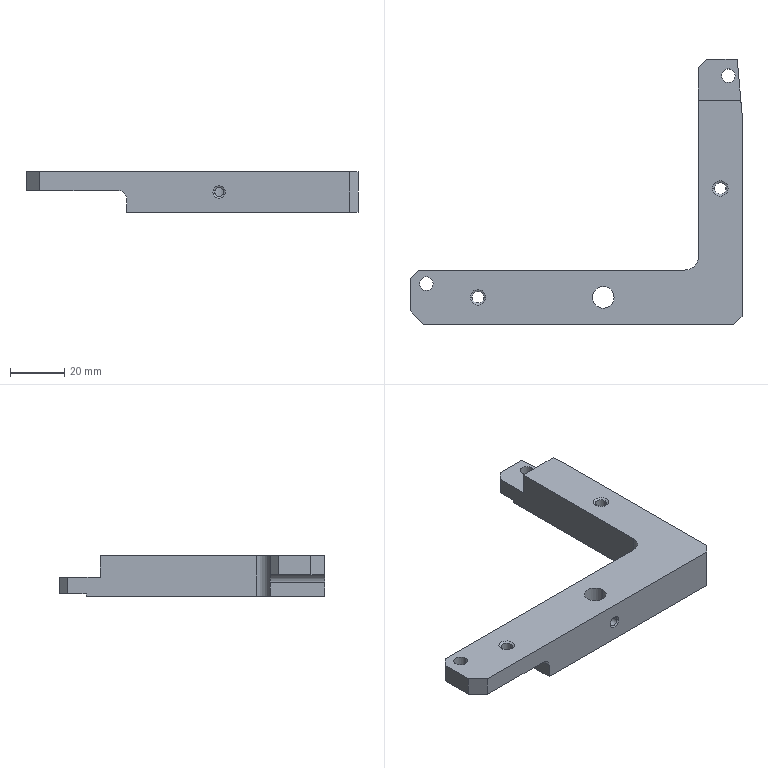Part | NX | 1 solid | 39 faces | box 122 x 97.43 x 15 mm | volume 45601 mm3 | plane 19 | cylinder 14 | cone 6 | commonest cylinder face diameters 4.2 x4 5 x4 3.3 x2 8 x2 6 x1 10 x1
STEP:
#1=CARTESIAN_POINT('',(-61.,7.,0.5));
#2=VERTEX_POINT('',#1);
#3=CARTESIAN_POINT('',(-61.,-5.,0.5));
#4=VERTEX_POINT('',#3);
#5=CARTESIAN_POINT('',(-61.,0.,0.5));
#6=DIRECTION('',(0.,-1.,0.));
#7=VECTOR('',#6,1000.);
#8=LINE('',#5,#7);
#9=EDGE_CURVE('',#2,#4,#8,.T.);
#10=ORIENTED_EDGE('',*,*,#9,.F.);
#11=CARTESIAN_POINT('',(-58.,10.,0.5));
#12=VERTEX_POINT('',#11);
#13=CARTESIAN_POINT('',(-68.,0.,0.5));
#14=DIRECTION('',(-0.7071,-0.7071,0.));
#15=VECTOR('',#14,1000.);
#16=LINE('',#13,#15);
#17=EDGE_CURVE('',#12,#2,#16,.T.);
#18=ORIENTED_EDGE('',*,*,#17,.F.);
#19=CARTESIAN_POINT('',(-27.,10.,0.5));
#20=VERTEX_POINT('',#19);
#21=CARTESIAN_POINT('',(0.,10.,0.5));
#22=DIRECTION('',(-1.,0.,0.));
#23=VECTOR('',#22,1000.);
#24=LINE('',#21,#23);
#25=EDGE_CURVE('',#20,#12,#24,.T.);
#26=ORIENTED_EDGE('',*,*,#25,.F.);
#27=CARTESIAN_POINT('',(-27.,-10.,0.5));
#28=VERTEX_POINT('',#27);
#29=CARTESIAN_POINT('',(-27.,10.,0.5));
#30=DIRECTION('',(0.,-1.,0.));
#31=VECTOR('',#30,1000.);
#32=LINE('',#29,#31);
#33=EDGE_CURVE('',#20,#28,#32,.T.);
#34=ORIENTED_EDGE('',*,*,#33,.T.);
#35=CARTESIAN_POINT('',(-56.,-10.,0.5));
#36=VERTEX_POINT('',#35);
#37=CARTESIAN_POINT('',(0.,-10.,0.5));
#38=DIRECTION('',(1.,0.,0.));
#39=VECTOR('',#38,1000.);
#40=LINE('',#37,#39);
#41=EDGE_CURVE('',#36,#28,#40,.T.);
#42=ORIENTED_EDGE('',*,*,#41,.F.);
#43=CARTESIAN_POINT('',(-66.,0.,0.5));
#44=DIRECTION('',(0.7071,-0.7071,0.));
#45=VECTOR('',#44,1000.);
#46=LINE('',#43,#45);
#47=EDGE_CURVE('',#4,#36,#46,.T.);
#48=ORIENTED_EDGE('',*,*,#47,.F.);
#49=EDGE_LOOP('',(#10,#18,#26,#34,#42,#48));
#50=FACE_BOUND('',#49,.T.);
#51=CARTESIAN_POINT('',(-52.5,5.,0.5));
#52=VERTEX_POINT('',#51);
#53=CARTESIAN_POINT('',(-57.5,5.,0.5));
#54=VERTEX_POINT('',#53);
#55=CARTESIAN_POINT('',(-55.,5.,0.5));
#56=DIRECTION('',(0.,0.,-1.));
#57=DIRECTION('',(-1.,0.,0.));
#58=AXIS2_PLACEMENT_3D('',#55,#56,#57);
#59=CIRCLE('',#58,2.5);
#60=EDGE_CURVE('',#52,#54,#59,.T.);
#61=ORIENTED_EDGE('',*,*,#60,.F.);
#62=CARTESIAN_POINT('',(-55.,5.,0.5));
#63=DIRECTION('',(0.,0.,-1.));
#64=DIRECTION('',(-1.,0.,0.));
#65=AXIS2_PLACEMENT_3D('',#62,#63,#64);
#66=CIRCLE('',#65,2.5);
#67=EDGE_CURVE('',#54,#52,#66,.T.);
#68=ORIENTED_EDGE('',*,*,#67,.F.);
#69=EDGE_LOOP('',(#61,#68));
#70=FACE_BOUND('',#69,.T.);
#71=CARTESIAN_POINT('',(-33.9,0.,0.5));
#72=VERTEX_POINT('',#71);
#73=CARTESIAN_POINT('',(-38.1,0.,0.5));
#74=VERTEX_POINT('',#73);
#75=CARTESIAN_POINT('',(-36.,0.,0.5));
#76=DIRECTION('',(0.,0.,1.));
#77=DIRECTION('',(1.,0.,0.));
#78=AXIS2_PLACEMENT_3D('',#75,#76,#77);
#79=CIRCLE('',#78,2.1);
#80=EDGE_CURVE('',#72,#74,#79,.T.);
#81=ORIENTED_EDGE('',*,*,#80,.T.);
#82=CARTESIAN_POINT('',(-36.,0.,0.5));
#83=DIRECTION('',(0.,0.,1.));
#84=DIRECTION('',(1.,0.,0.));
#85=AXIS2_PLACEMENT_3D('',#82,#83,#84);
#86=CIRCLE('',#85,2.1);
#87=EDGE_CURVE('',#74,#72,#86,.T.);
#88=ORIENTED_EDGE('',*,*,#87,.T.);
#89=EDGE_LOOP('',(#81,#88));
#90=FACE_BOUND('',#89,.T.);
#91=CARTESIAN_POINT('',(-61.,10.,0.5));
#92=DIRECTION('',(0.,0.,1.));
#93=DIRECTION('',(1.,0.,0.));
#94=AXIS2_PLACEMENT_3D('',#91,#92,#93);
#95=PLANE('',#94);
#96=ADVANCED_FACE('',(#50,#70,#90),#95,.F.);
#97=CARTESIAN_POINT('',(60.108,77.63,-7.5));
#98=VERTEX_POINT('',#97);
#99=CARTESIAN_POINT('',(45.,77.63,-7.5));
#100=VERTEX_POINT('',#99);
#101=CARTESIAN_POINT('',(0.,77.63,-7.5));
#102=DIRECTION('',(-1.,0.,0.));
#103=VECTOR('',#102,1000.);
#104=LINE('',#101,#103);
#105=EDGE_CURVE('',#98,#100,#104,.T.);
#106=ORIENTED_EDGE('',*,*,#105,.T.);
#107=CARTESIAN_POINT('',(45.,77.63,-6.5));
#108=VERTEX_POINT('',#107);
#109=CARTESIAN_POINT('',(45.,77.63,-6.5));
#110=DIRECTION('',(0.,0.,-1.));
#111=VECTOR('',#110,1000.);
#112=LINE('',#109,#111);
#113=EDGE_CURVE('',#108,#100,#112,.T.);
#114=ORIENTED_EDGE('',*,*,#113,.F.);
#115=CARTESIAN_POINT('',(60.108,77.63,-6.5));
#116=VERTEX_POINT('',#115);
#117=CARTESIAN_POINT('',(45.,77.63,-6.5));
#118=DIRECTION('',(1.,0.,0.));
#119=VECTOR('',#118,1000.);
#120=LINE('',#117,#119);
#121=EDGE_CURVE('',#108,#116,#120,.T.);
#122=ORIENTED_EDGE('',*,*,#121,.T.);
#123=CARTESIAN_POINT('',(60.108,77.63,-6.5));
#124=DIRECTION('',(0.,0.,-1.));
#125=VECTOR('',#124,1000.);
#126=LINE('',#123,#125);
#127=EDGE_CURVE('',#116,#98,#126,.T.);
#128=ORIENTED_EDGE('',*,*,#127,.T.);
#129=EDGE_LOOP('',(#106,#114,#122,#128));
#130=FACE_BOUND('',#129,.T.);
#131=CARTESIAN_POINT('',(64.741,77.63,-7.5));
#132=DIRECTION('',(0.,-1.,0.));
#133=DIRECTION('',(0.,0.,-1.));
#134=AXIS2_PLACEMENT_3D('',#131,#132,#133);
#135=PLANE('',#134);
#136=ADVANCED_FACE('',(#130),#135,.F.);
#137=CARTESIAN_POINT('',(59.25,87.43,-6.5));
#138=VERTEX_POINT('',#137);
#139=CARTESIAN_POINT('',(60.108,77.63,-6.5));
#140=DIRECTION('',(-0.08716,0.9962,0.));
#141=VECTOR('',#140,1000.);
#142=LINE('',#139,#141);
#143=EDGE_CURVE('',#116,#138,#142,.T.);
#144=ORIENTED_EDGE('',*,*,#143,.T.);
#145=CARTESIAN_POINT('',(59.25,87.43,-0.5));
#146=VERTEX_POINT('',#145);
#147=CARTESIAN_POINT('',(59.25,87.43,-6.5));
#148=DIRECTION('',(0.,0.,1.));
#149=VECTOR('',#148,1000.);
#150=LINE('',#147,#149);
#151=EDGE_CURVE('',#138,#146,#150,.T.);
#152=ORIENTED_EDGE('',*,*,#151,.T.);
#153=CARTESIAN_POINT('',(60.563,72.43,-0.5));
#154=VERTEX_POINT('',#153);
#155=CARTESIAN_POINT('',(59.25,87.43,-0.5));
#156=DIRECTION('',(0.08716,-0.9962,0.));
#157=VECTOR('',#156,1000.);
#158=LINE('',#155,#157);
#159=EDGE_CURVE('',#146,#154,#158,.T.);
#160=ORIENTED_EDGE('',*,*,#159,.T.);
#161=CARTESIAN_POINT('',(60.563,72.43,7.5));
#162=VERTEX_POINT('',#161);
#163=CARTESIAN_POINT('',(60.563,72.43,7.5));
#164=DIRECTION('',(0.,0.,-1.));
#165=VECTOR('',#164,1000.);
#166=LINE('',#163,#165);
#167=EDGE_CURVE('',#162,#154,#166,.T.);
#168=ORIENTED_EDGE('',*,*,#167,.F.);
#169=CARTESIAN_POINT('',(61.,67.43,7.5));
#170=VERTEX_POINT('',#169);
#171=CARTESIAN_POINT('',(66.899,0.,7.5));
#172=DIRECTION('',(-0.08716,0.9962,0.));
#173=VECTOR('',#172,1000.);
#174=LINE('',#171,#173);
#175=EDGE_CURVE('',#170,#162,#174,.T.);
#176=ORIENTED_EDGE('',*,*,#175,.F.);
#177=CARTESIAN_POINT('',(61.,67.43,-7.5));
#178=VERTEX_POINT('',#177);
#179=CARTESIAN_POINT('',(61.,67.43,7.5));
#180=DIRECTION('',(0.,0.,-1.));
#181=VECTOR('',#180,1000.);
#182=LINE('',#179,#181);
#183=EDGE_CURVE('',#170,#178,#182,.T.);
#184=ORIENTED_EDGE('',*,*,#183,.T.);
#185=CARTESIAN_POINT('',(66.899,0.,-7.5));
#186=DIRECTION('',(-0.08716,0.9962,0.));
#187=VECTOR('',#186,1000.);
#188=LINE('',#185,#187);
#189=EDGE_CURVE('',#178,#98,#188,.T.);
#190=ORIENTED_EDGE('',*,*,#189,.T.);
#191=ORIENTED_EDGE('',*,*,#127,.F.);
#192=EDGE_LOOP('',(#144,#152,#160,#168,#176,#184,#190,#191));
#193=FACE_BOUND('',#192,.T.);
#194=CARTESIAN_POINT('',(61.,67.43,-7.5));
#195=DIRECTION('',(-0.9962,-0.08716,0.));
#196=DIRECTION('',(-0.08716,0.9962,0.));
#197=AXIS2_PLACEMENT_3D('',#194,#195,#196);
#198=PLANE('',#197);
#199=ADVANCED_FACE('',(#193),#198,.F.);
#200=CARTESIAN_POINT('',(48.,87.43,-6.5));
#201=VERTEX_POINT('',#200);
#202=CARTESIAN_POINT('',(59.25,87.43,-6.5));
#203=DIRECTION('',(-1.,0.,0.));
#204=VECTOR('',#203,1000.);
#205=LINE('',#202,#204);
#206=EDGE_CURVE('',#138,#201,#205,.T.);
#207=ORIENTED_EDGE('',*,*,#206,.F.);
#208=ORIENTED_EDGE('',*,*,#143,.F.);
#209=ORIENTED_EDGE('',*,*,#121,.F.);
#210=CARTESIAN_POINT('',(45.,84.43,-6.5));
#211=VERTEX_POINT('',#210);
#212=CARTESIAN_POINT('',(45.,77.63,-6.5));
#213=DIRECTION('',(0.,1.,0.));
#214=VECTOR('',#213,1000.);
#215=LINE('',#212,#214);
#216=EDGE_CURVE('',#108,#211,#215,.T.);
#217=ORIENTED_EDGE('',*,*,#216,.T.);
#218=CARTESIAN_POINT('',(48.,87.43,-6.5));
#219=DIRECTION('',(-0.7071,-0.7071,0.));
#220=VECTOR('',#219,1000.);
#221=LINE('',#218,#220);
#222=EDGE_CURVE('',#201,#211,#221,.T.);
#223=ORIENTED_EDGE('',*,*,#222,.F.);
#224=EDGE_LOOP('',(#207,#208,#209,#217,#223));
#225=FACE_BOUND('',#224,.T.);
#226=CARTESIAN_POINT('',(53.5,81.43,-6.5));
#227=VERTEX_POINT('',#226);
#228=CARTESIAN_POINT('',(58.5,81.43,-6.5));
#229=VERTEX_POINT('',#228);
#230=CARTESIAN_POINT('',(56.,81.43,-6.5));
#231=DIRECTION('',(0.,0.,-1.));
#232=DIRECTION('',(1.,0.,0.));
#233=AXIS2_PLACEMENT_3D('',#230,#231,#232);
#234=CIRCLE('',#233,2.5);
#235=EDGE_CURVE('',#227,#229,#234,.T.);
#236=ORIENTED_EDGE('',*,*,#235,.F.);
#237=CARTESIAN_POINT('',(56.,81.43,-6.5));
#238=DIRECTION('',(0.,0.,-1.));
#239=DIRECTION('',(1.,0.,0.));
#240=AXIS2_PLACEMENT_3D('',#237,#238,#239);
#241=CIRCLE('',#240,2.5);
#242=EDGE_CURVE('',#229,#227,#241,.T.);
#243=ORIENTED_EDGE('',*,*,#242,.F.);
#244=EDGE_LOOP('',(#236,#243));
#245=FACE_BOUND('',#244,.T.);
#246=CARTESIAN_POINT('',(0.,0.,-6.5));
#247=DIRECTION('',(0.,0.,-1.));
#248=DIRECTION('',(0.,-1.,0.));
#249=AXIS2_PLACEMENT_3D('',#246,#247,#248);
#250=PLANE('',#249);
#251=ADVANCED_FACE('',(#225,#245),#250,.T.);
#252=ORIENTED_EDGE('',*,*,#206,.T.);
#253=CARTESIAN_POINT('',(48.,87.43,-0.5));
#254=VERTEX_POINT('',#253);
#255=CARTESIAN_POINT('',(48.,87.43,-0.5));
#256=DIRECTION('',(0.,0.,-1.));
#257=VECTOR('',#256,1000.);
#258=LINE('',#255,#257);
#259=EDGE_CURVE('',#254,#201,#258,.T.);
#260=ORIENTED_EDGE('',*,*,#259,.F.);
#261=CARTESIAN_POINT('',(59.25,87.43,-0.5));
#262=DIRECTION('',(-1.,0.,0.));
#263=VECTOR('',#262,1000.);
#264=LINE('',#261,#263);
#265=EDGE_CURVE('',#146,#254,#264,.T.);
#266=ORIENTED_EDGE('',*,*,#265,.F.);
#267=ORIENTED_EDGE('',*,*,#151,.F.);
#268=EDGE_LOOP('',(#252,#260,#266,#267));
#269=FACE_BOUND('',#268,.T.);
#270=CARTESIAN_POINT('',(0.,87.43,-7.5));
#271=DIRECTION('',(0.,1.,0.));
#272=DIRECTION('',(1.,0.,0.));
#273=AXIS2_PLACEMENT_3D('',#270,#271,#272);
#274=PLANE('',#273);
#275=ADVANCED_FACE('',(#269),#274,.T.);
#276=CARTESIAN_POINT('',(45.,72.43,-0.5));
#277=VERTEX_POINT('',#276);
#278=CARTESIAN_POINT('',(60.563,72.43,-0.5));
#279=DIRECTION('',(-1.,0.,0.));
#280=VECTOR('',#279,1000.);
#281=LINE('',#278,#280);
#282=EDGE_CURVE('',#154,#277,#281,.T.);
#283=ORIENTED_EDGE('',*,*,#282,.F.);
#284=ORIENTED_EDGE('',*,*,#159,.F.);
#285=ORIENTED_EDGE('',*,*,#265,.T.);
#286=CARTESIAN_POINT('',(45.,84.43,-0.5));
#287=VERTEX_POINT('',#286);
#288=CARTESIAN_POINT('',(45.,84.43,-0.5));
#289=DIRECTION('',(0.7071,0.7071,0.));
#290=VECTOR('',#289,1000.);
#291=LINE('',#288,#290);
#292=EDGE_CURVE('',#287,#254,#291,.T.);
#293=ORIENTED_EDGE('',*,*,#292,.F.);
#294=CARTESIAN_POINT('',(45.,72.43,-0.5));
#295=DIRECTION('',(0.,1.,0.));
#296=VECTOR('',#295,1000.);
#297=LINE('',#294,#296);
#298=EDGE_CURVE('',#277,#287,#297,.T.);
#299=ORIENTED_EDGE('',*,*,#298,.F.);
#300=EDGE_LOOP('',(#283,#284,#285,#293,#299));
#301=FACE_BOUND('',#300,.T.);
#302=CARTESIAN_POINT('',(58.5,81.43,-0.5));
#303=VERTEX_POINT('',#302);
#304=CARTESIAN_POINT('',(53.5,81.43,-0.5));
#305=VERTEX_POINT('',#304);
#306=CARTESIAN_POINT('',(56.,81.43,-0.5));
#307=DIRECTION('',(0.,0.,1.));
#308=DIRECTION('',(-1.,0.,0.));
#309=AXIS2_PLACEMENT_3D('',#306,#307,#308);
#310=CIRCLE('',#309,2.5);
#311=EDGE_CURVE('',#303,#305,#310,.T.);
#312=ORIENTED_EDGE('',*,*,#311,.F.);
#313=CARTESIAN_POINT('',(56.,81.43,-0.5));
#314=DIRECTION('',(0.,0.,1.));
#315=DIRECTION('',(-1.,0.,0.));
#316=AXIS2_PLACEMENT_3D('',#313,#314,#315);
#317=CIRCLE('',#316,2.5);
#318=EDGE_CURVE('',#305,#303,#317,.T.);
#319=ORIENTED_EDGE('',*,*,#318,.F.);
#320=EDGE_LOOP('',(#312,#319));
#321=FACE_BOUND('',#320,.T.);
#322=CARTESIAN_POINT('',(45.,87.43,-0.5));
#323=DIRECTION('',(0.,0.,-1.));
#324=DIRECTION('',(0.,-1.,0.));
#325=AXIS2_PLACEMENT_3D('',#322,#323,#324);
#326=PLANE('',#325);
#327=ADVANCED_FACE('',(#301,#321),#326,.F.);
#328=ORIENTED_EDGE('',*,*,#282,.T.);
#329=CARTESIAN_POINT('',(45.,72.43,7.5));
#330=VERTEX_POINT('',#329);
#331=CARTESIAN_POINT('',(45.,72.43,-0.5));
#332=DIRECTION('',(0.,0.,1.));
#333=VECTOR('',#332,1000.);
#334=LINE('',#331,#333);
#335=EDGE_CURVE('',#277,#330,#334,.T.);
#336=ORIENTED_EDGE('',*,*,#335,.T.);
#337=CARTESIAN_POINT('',(0.,72.43,7.5));
#338=DIRECTION('',(-1.,0.,0.));
#339=VECTOR('',#338,1000.);
#340=LINE('',#337,#339);
#341=EDGE_CURVE('',#162,#330,#340,.T.);
#342=ORIENTED_EDGE('',*,*,#341,.F.);
#343=ORIENTED_EDGE('',*,*,#167,.T.);
#344=EDGE_LOOP('',(#328,#336,#342,#343));
#345=FACE_BOUND('',#344,.T.);
#346=CARTESIAN_POINT('',(45.,72.43,-0.5));
#347=DIRECTION('',(0.,-1.,0.));
#348=DIRECTION('',(0.,0.,-1.));
#349=AXIS2_PLACEMENT_3D('',#346,#347,#348);
#350=PLANE('',#349);
#351=ADVANCED_FACE('',(#345),#350,.F.);
#352=ORIENTED_EDGE('',*,*,#105,.F.);
#353=ORIENTED_EDGE('',*,*,#189,.F.);
#354=CARTESIAN_POINT('',(61.,-7.,-7.5));
#355=VERTEX_POINT('',#354);
#356=CARTESIAN_POINT('',(61.,0.,-7.5));
#357=DIRECTION('',(0.,-1.,0.));
#358=VECTOR('',#357,1000.);
#359=LINE('',#356,#358);
#360=EDGE_CURVE('',#178,#355,#359,.T.);
#361=ORIENTED_EDGE('',*,*,#360,.T.);
#362=CARTESIAN_POINT('',(58.,-10.,-7.5));
#363=VERTEX_POINT('',#362);
#364=CARTESIAN_POINT('',(68.,0.,-7.5));
#365=DIRECTION('',(0.7071,0.7071,0.));
#366=VECTOR('',#365,1000.);
#367=LINE('',#364,#366);
#368=EDGE_CURVE('',#363,#355,#367,.T.);
#369=ORIENTED_EDGE('',*,*,#368,.F.);
#370=CARTESIAN_POINT('',(-24.,-10.,-7.5));
#371=VERTEX_POINT('',#370);
#372=CARTESIAN_POINT('',(0.,-10.,-7.5));
#373=DIRECTION('',(1.,0.,0.));
#374=VECTOR('',#373,1000.);
#375=LINE('',#372,#374);
#376=EDGE_CURVE('',#371,#363,#375,.T.);
#377=ORIENTED_EDGE('',*,*,#376,.F.);
#378=CARTESIAN_POINT('',(-24.,10.,-7.5));
#379=VERTEX_POINT('',#378);
#380=CARTESIAN_POINT('',(-24.,0.,-7.5));
#381=DIRECTION('',(0.,-1.,0.));
#382=VECTOR('',#381,1000.);
#383=LINE('',#380,#382);
#384=EDGE_CURVE('',#379,#371,#383,.T.);
#385=ORIENTED_EDGE('',*,*,#384,.F.);
#386=CARTESIAN_POINT('',(40.,10.,-7.5));
#387=VERTEX_POINT('',#386);
#388=CARTESIAN_POINT('',(0.,10.,-7.5));
#389=DIRECTION('',(1.,0.,0.));
#390=VECTOR('',#389,1000.);
#391=LINE('',#388,#390);
#392=EDGE_CURVE('',#379,#387,#391,.T.);
#393=ORIENTED_EDGE('',*,*,#392,.T.);
#394=CARTESIAN_POINT('',(45.,15.,-7.5));
#395=VERTEX_POINT('',#394);
#396=CARTESIAN_POINT('',(40.,15.,-7.5));
#397=DIRECTION('',(0.,0.,1.));
#398=DIRECTION('',(0.,-1.,0.));
#399=AXIS2_PLACEMENT_3D('',#396,#397,#398);
#400=CIRCLE('',#399,5.);
#401=EDGE_CURVE('',#387,#395,#400,.T.);
#402=ORIENTED_EDGE('',*,*,#401,.T.);
#403=CARTESIAN_POINT('',(45.,0.,-7.5));
#404=DIRECTION('',(0.,1.,0.));
#405=VECTOR('',#404,1000.);
#406=LINE('',#403,#405);
#407=EDGE_CURVE('',#395,#100,#406,.T.);
#408=ORIENTED_EDGE('',*,*,#407,.T.);
#409=EDGE_LOOP('',(#352,#353,#361,#369,#377,#385,#393,#402,#408));
#410=FACE_BOUND('',#409,.T.);
#411=CARTESIAN_POINT('',(6.,0.,-7.5));
#412=VERTEX_POINT('',#411);
#413=CARTESIAN_POINT('',(14.,0.,-7.5));
#414=VERTEX_POINT('',#413);
#415=CARTESIAN_POINT('',(10.,0.,-7.5));
#416=DIRECTION('',(0.,0.,-1.));
#417=DIRECTION('',(-1.,0.,0.));
#418=AXIS2_PLACEMENT_3D('',#415,#416,#417);
#419=CIRCLE('',#418,4.);
#420=EDGE_CURVE('',#412,#414,#419,.T.);
#421=ORIENTED_EDGE('',*,*,#420,.F.);
#422=CARTESIAN_POINT('',(10.,0.,-7.5));
#423=DIRECTION('',(0.,0.,-1.));
#424=DIRECTION('',(-1.,0.,0.));
#425=AXIS2_PLACEMENT_3D('',#422,#423,#424);
#426=CIRCLE('',#425,4.);
#427=EDGE_CURVE('',#414,#412,#426,.T.);
#428=ORIENTED_EDGE('',*,*,#427,.F.);
#429=EDGE_LOOP('',(#421,#428));
#430=FACE_BOUND('',#429,.T.);
#431=CARTESIAN_POINT('',(50.9,40.,-7.5));
#432=VERTEX_POINT('',#431);
#433=CARTESIAN_POINT('',(55.1,40.,-7.5));
#434=VERTEX_POINT('',#433);
#435=CARTESIAN_POINT('',(53.,40.,-7.5));
#436=DIRECTION('',(0.,0.,1.));
#437=DIRECTION('',(1.,0.,0.));
#438=AXIS2_PLACEMENT_3D('',#435,#436,#437);
#439=CIRCLE('',#438,2.1);
#440=EDGE_CURVE('',#432,#434,#439,.T.);
#441=ORIENTED_EDGE('',*,*,#440,.T.);
#442=CARTESIAN_POINT('',(53.,40.,-7.5));
#443=DIRECTION('',(0.,0.,1.));
#444=DIRECTION('',(1.,0.,0.));
#445=AXIS2_PLACEMENT_3D('',#442,#443,#444);
#446=CIRCLE('',#445,2.1);
#447=EDGE_CURVE('',#434,#432,#446,.T.);
#448=ORIENTED_EDGE('',*,*,#447,.T.);
#449=EDGE_LOOP('',(#441,#448));
#450=FACE_BOUND('',#449,.T.);
#451=CARTESIAN_POINT('',(0.,0.,-7.5));
#452=DIRECTION('',(0.,0.,1.));
#453=DIRECTION('',(1.,0.,0.));
#454=AXIS2_PLACEMENT_3D('',#451,#452,#453);
#455=PLANE('',#454);
#456=ADVANCED_FACE('',(#410,#430,#450),#455,.F.);
#457=CARTESIAN_POINT('',(61.,-7.,7.5));
#458=VERTEX_POINT('',#457);
#459=CARTESIAN_POINT('',(61.,-7.,0.));
#460=DIRECTION('',(0.,0.,-1.));
#461=VECTOR('',#460,1000.);
#462=LINE('',#459,#461);
#463=EDGE_CURVE('',#458,#355,#462,.T.);
#464=ORIENTED_EDGE('',*,*,#463,.T.);
#465=ORIENTED_EDGE('',*,*,#360,.F.);
#466=ORIENTED_EDGE('',*,*,#183,.F.);
#467=CARTESIAN_POINT('',(61.,0.,7.5));
#468=DIRECTION('',(0.,-1.,0.));
#469=VECTOR('',#468,1000.);
#470=LINE('',#467,#469);
#471=EDGE_CURVE('',#170,#458,#470,.T.);
#472=ORIENTED_EDGE('',*,*,#471,.T.);
#473=EDGE_LOOP('',(#464,#465,#466,#472));
#474=FACE_BOUND('',#473,.T.);
#475=CARTESIAN_POINT('',(61.,-10.,-7.5));
#476=DIRECTION('',(1.,0.,0.));
#477=DIRECTION('',(0.,1.,0.));
#478=AXIS2_PLACEMENT_3D('',#475,#476,#477);
#479=PLANE('',#478);
#480=ADVANCED_FACE('',(#474),#479,.T.);
#481=CARTESIAN_POINT('',(-56.,-10.,7.5));
#482=VERTEX_POINT('',#481);
#483=CARTESIAN_POINT('',(58.,-10.,7.5));
#484=VERTEX_POINT('',#483);
#485=CARTESIAN_POINT('',(0.,-10.,7.5));
#486=DIRECTION('',(1.,0.,0.));
#487=VECTOR('',#486,1000.);
#488=LINE('',#485,#487);
#489=EDGE_CURVE('',#482,#484,#488,.T.);
#490=ORIENTED_EDGE('',*,*,#489,.T.);
#491=CARTESIAN_POINT('',(68.,0.,7.5));
#492=DIRECTION('',(0.7071,0.7071,0.));
#493=VECTOR('',#492,1000.);
#494=LINE('',#491,#493);
#495=EDGE_CURVE('',#484,#458,#494,.T.);
#496=ORIENTED_EDGE('',*,*,#495,.T.);
#497=ORIENTED_EDGE('',*,*,#471,.F.);
#498=ORIENTED_EDGE('',*,*,#175,.T.);
#499=ORIENTED_EDGE('',*,*,#341,.T.);
#500=CARTESIAN_POINT('',(45.,15.,7.5));
#501=VERTEX_POINT('',#500);
#502=CARTESIAN_POINT('',(45.,0.,7.5));
#503=DIRECTION('',(0.,1.,0.));
#504=VECTOR('',#503,1000.);
#505=LINE('',#502,#504);
#506=EDGE_CURVE('',#501,#330,#505,.T.);
#507=ORIENTED_EDGE('',*,*,#506,.F.);
#508=CARTESIAN_POINT('',(40.,10.,7.5));
#509=VERTEX_POINT('',#508);
#510=CARTESIAN_POINT('',(40.,15.,7.5));
#511=DIRECTION('',(0.,0.,1.));
#512=DIRECTION('',(0.,-1.,0.));
#513=AXIS2_PLACEMENT_3D('',#510,#511,#512);
#514=CIRCLE('',#513,5.);
#515=EDGE_CURVE('',#509,#501,#514,.T.);
#516=ORIENTED_EDGE('',*,*,#515,.F.);
#517=CARTESIAN_POINT('',(-58.,10.,7.5));
#518=VERTEX_POINT('',#517);
#519=CARTESIAN_POINT('',(0.,10.,7.5));
#520=DIRECTION('',(1.,0.,0.));
#521=VECTOR('',#520,1000.);
#522=LINE('',#519,#521);
#523=EDGE_CURVE('',#518,#509,#522,.T.);
#524=ORIENTED_EDGE('',*,*,#523,.F.);
#525=CARTESIAN_POINT('',(-61.,7.,7.5));
#526=VERTEX_POINT('',#525);
#527=CARTESIAN_POINT('',(-68.,0.,7.5));
#528=DIRECTION('',(0.7071,0.7071,0.));
#529=VECTOR('',#528,1000.);
#530=LINE('',#527,#529);
#531=EDGE_CURVE('',#526,#518,#530,.T.);
#532=ORIENTED_EDGE('',*,*,#531,.F.);
#533=CARTESIAN_POINT('',(-61.,-5.,7.5));
#534=VERTEX_POINT('',#533);
#535=CARTESIAN_POINT('',(-61.,0.,7.5));
#536=DIRECTION('',(0.,1.,0.));
#537=VECTOR('',#536,1000.);
#538=LINE('',#535,#537);
#539=EDGE_CURVE('',#534,#526,#538,.T.);
#540=ORIENTED_EDGE('',*,*,#539,.F.);
#541=CARTESIAN_POINT('',(-66.,0.,7.5));
#542=DIRECTION('',(-0.7071,0.7071,0.));
#543=VECTOR('',#542,1000.);
#544=LINE('',#541,#543);
#545=EDGE_CURVE('',#482,#534,#544,.T.);
#546=ORIENTED_EDGE('',*,*,#545,.F.);
#547=EDGE_LOOP('',(#490,#496,#497,#498,#499,#507,#516,#524,#532,#540,#546));
#548=FACE_BOUND('',#547,.T.);
#549=CARTESIAN_POINT('',(-57.5,5.,7.5));
#550=VERTEX_POINT('',#549);
#551=CARTESIAN_POINT('',(-52.5,5.,7.5));
#552=VERTEX_POINT('',#551);
#553=CARTESIAN_POINT('',(-55.,5.,7.5));
#554=DIRECTION('',(0.,0.,-1.));
#555=DIRECTION('',(-1.,0.,0.));
#556=AXIS2_PLACEMENT_3D('',#553,#554,#555);
#557=CIRCLE('',#556,2.5);
#558=EDGE_CURVE('',#550,#552,#557,.T.);
#559=ORIENTED_EDGE('',*,*,#558,.T.);
#560=CARTESIAN_POINT('',(-55.,5.,7.5));
#561=DIRECTION('',(0.,0.,-1.));
#562=DIRECTION('',(-1.,0.,0.));
#563=AXIS2_PLACEMENT_3D('',#560,#561,#562);
#564=CIRCLE('',#563,2.5);
#565=EDGE_CURVE('',#552,#550,#564,.T.);
#566=ORIENTED_EDGE('',*,*,#565,.T.);
#567=EDGE_LOOP('',(#559,#566));
#568=FACE_BOUND('',#567,.T.);
#569=CARTESIAN_POINT('',(55.86,40.,7.5));
#570=VERTEX_POINT('',#569);
#571=CARTESIAN_POINT('',(50.14,40.,7.5));
#572=VERTEX_POINT('',#571);
#573=CARTESIAN_POINT('',(53.,40.,7.5));
#574=DIRECTION('',(0.,0.,1.));
#575=DIRECTION('',(1.,0.,0.));
#576=AXIS2_PLACEMENT_3D('',#573,#574,#575);
#577=CIRCLE('',#576,2.86);
#578=EDGE_CURVE('',#570,#572,#577,.T.);
#579=ORIENTED_EDGE('',*,*,#578,.F.);
#580=CARTESIAN_POINT('',(53.,40.,7.5));
#581=DIRECTION('',(0.,0.,1.));
#582=DIRECTION('',(1.,0.,0.));
#583=AXIS2_PLACEMENT_3D('',#580,#581,#582);
#584=CIRCLE('',#583,2.86);
#585=EDGE_CURVE('',#572,#570,#584,.T.);
#586=ORIENTED_EDGE('',*,*,#585,.F.);
#587=EDGE_LOOP('',(#579,#586));
#588=FACE_BOUND('',#587,.T.);
#589=CARTESIAN_POINT('',(-38.86,0.,7.5));
#590=VERTEX_POINT('',#589);
#591=CARTESIAN_POINT('',(-33.14,0.,7.5));
#592=VERTEX_POINT('',#591);
#593=CARTESIAN_POINT('',(-36.,0.,7.5));
#594=DIRECTION('',(0.,0.,1.));
#595=DIRECTION('',(1.,0.,0.));
#596=AXIS2_PLACEMENT_3D('',#593,#594,#595);
#597=CIRCLE('',#596,2.86);
#598=EDGE_CURVE('',#590,#592,#597,.T.);
#599=ORIENTED_EDGE('',*,*,#598,.F.);
#600=CARTESIAN_POINT('',(-36.,0.,7.5));
#601=DIRECTION('',(0.,0.,1.));
#602=DIRECTION('',(1.,0.,0.));
#603=AXIS2_PLACEMENT_3D('',#600,#601,#602);
#604=CIRCLE('',#603,2.86);
#605=EDGE_CURVE('',#592,#590,#604,.T.);
#606=ORIENTED_EDGE('',*,*,#605,.F.);
#607=EDGE_LOOP('',(#599,#606));
#608=FACE_BOUND('',#607,.T.);
#609=CARTESIAN_POINT('',(14.,0.,7.5));
#610=VERTEX_POINT('',#609);
#611=CARTESIAN_POINT('',(6.,0.,7.5));
#612=VERTEX_POINT('',#611);
#613=CARTESIAN_POINT('',(10.,0.,7.5));
#614=DIRECTION('',(0.,0.,-1.));
#615=DIRECTION('',(-1.,0.,0.));
#616=AXIS2_PLACEMENT_3D('',#613,#614,#615);
#617=CIRCLE('',#616,4.);
#618=EDGE_CURVE('',#610,#612,#617,.T.);
#619=ORIENTED_EDGE('',*,*,#618,.T.);
#620=CARTESIAN_POINT('',(10.,0.,7.5));
#621=DIRECTION('',(0.,0.,-1.));
#622=DIRECTION('',(-1.,0.,0.));
#623=AXIS2_PLACEMENT_3D('',#620,#621,#622);
#624=CIRCLE('',#623,4.);
#625=EDGE_CURVE('',#612,#610,#624,.T.);
#626=ORIENTED_EDGE('',*,*,#625,.T.);
#627=EDGE_LOOP('',(#619,#626));
#628=FACE_BOUND('',#627,.T.);
#629=CARTESIAN_POINT('',(0.,0.,7.5));
#630=DIRECTION('',(0.,0.,1.));
#631=DIRECTION('',(1.,0.,0.));
#632=AXIS2_PLACEMENT_3D('',#629,#630,#631);
#633=PLANE('',#632);
#634=ADVANCED_FACE('',(#548,#568,#588,#608,#628),#633,.T.);
#635=CARTESIAN_POINT('',(-24.,10.,-2.5));
#636=VERTEX_POINT('',#635);
#637=CARTESIAN_POINT('',(-24.,-10.,-2.5));
#638=VERTEX_POINT('',#637);
#639=CARTESIAN_POINT('',(-24.,10.245,-2.5));
#640=DIRECTION('',(0.,-1.,0.));
#641=VECTOR('',#640,1000.);
#642=LINE('',#639,#641);
#643=EDGE_CURVE('',#636,#638,#642,.T.);
#644=ORIENTED_EDGE('',*,*,#643,.F.);
#645=CARTESIAN_POINT('',(-24.,10.,-2.5));
#646=DIRECTION('',(0.,0.,-1.));
#647=VECTOR('',#646,1000.);
#648=LINE('',#645,#647);
#649=EDGE_CURVE('',#636,#379,#648,.T.);
#650=ORIENTED_EDGE('',*,*,#649,.T.);
#651=ORIENTED_EDGE('',*,*,#384,.T.);
#652=CARTESIAN_POINT('',(-24.,-10.,0.));
#653=DIRECTION('',(0.,0.,-1.));
#654=VECTOR('',#653,1000.);
#655=LINE('',#652,#654);
#656=EDGE_CURVE('',#638,#371,#655,.T.);
#657=ORIENTED_EDGE('',*,*,#656,.F.);
#658=EDGE_LOOP('',(#644,#650,#651,#657));
#659=FACE_BOUND('',#658,.T.);
#660=CARTESIAN_POINT('',(-24.,10.,0.5));
#661=DIRECTION('',(1.,0.,0.));
#662=DIRECTION('',(0.,1.,0.));
#663=AXIS2_PLACEMENT_3D('',#660,#661,#662);
#664=PLANE('',#663);
#665=ADVANCED_FACE('',(#659),#664,.F.);
#666=ORIENTED_EDGE('',*,*,#643,.T.);
#667=CARTESIAN_POINT('',(-27.,-10.,-2.5));
#668=DIRECTION('',(0.,-1.,0.));
#669=DIRECTION('',(1.,0.,0.));
#670=AXIS2_PLACEMENT_3D('',#667,#668,#669);
#671=CIRCLE('',#670,3.);
#672=EDGE_CURVE('',#638,#28,#671,.T.);
#673=ORIENTED_EDGE('',*,*,#672,.T.);
#674=ORIENTED_EDGE('',*,*,#33,.F.);
#675=CARTESIAN_POINT('',(-27.,10.,-2.5));
#676=DIRECTION('',(0.,1.,0.));
#677=DIRECTION('',(0.,0.,1.));
#678=AXIS2_PLACEMENT_3D('',#675,#676,#677);
#679=CIRCLE('',#678,3.);
#680=EDGE_CURVE('',#20,#636,#679,.T.);
#681=ORIENTED_EDGE('',*,*,#680,.T.);
#682=EDGE_LOOP('',(#666,#673,#674,#681));
#683=FACE_BOUND('',#682,.T.);
#684=CARTESIAN_POINT('',(-27.,10.245,-2.5));
#685=DIRECTION('',(0.,-1.,0.));
#686=DIRECTION('',(1.,0.,0.));
#687=AXIS2_PLACEMENT_3D('',#684,#685,#686);
#688=CYLINDRICAL_SURFACE('',#687,3.);
#689=ADVANCED_FACE('',(#683),#688,.F.);
#690=ORIENTED_EDGE('',*,*,#25,.T.);
#691=CARTESIAN_POINT('',(-58.,10.,7.5));
#692=DIRECTION('',(0.,0.,-1.));
#693=VECTOR('',#692,1000.);
#694=LINE('',#691,#693);
#695=EDGE_CURVE('',#518,#12,#694,.T.);
#696=ORIENTED_EDGE('',*,*,#695,.F.);
#697=ORIENTED_EDGE('',*,*,#523,.T.);
#698=CARTESIAN_POINT('',(40.,10.,-7.737));
#699=DIRECTION('',(0.,0.,1.));
#700=VECTOR('',#699,1000.);
#701=LINE('',#698,#700);
#702=EDGE_CURVE('',#387,#509,#701,.T.);
#703=ORIENTED_EDGE('',*,*,#702,.F.);
#704=ORIENTED_EDGE('',*,*,#392,.F.);
#705=ORIENTED_EDGE('',*,*,#649,.F.);
#706=ORIENTED_EDGE('',*,*,#680,.F.);
#707=EDGE_LOOP('',(#690,#696,#697,#703,#704,#705,#706));
#708=FACE_BOUND('',#707,.T.);
#709=CARTESIAN_POINT('',(61.,10.,-7.5));
#710=DIRECTION('',(0.,1.,0.));
#711=DIRECTION('',(1.,0.,0.));
#712=AXIS2_PLACEMENT_3D('',#709,#710,#711);
#713=PLANE('',#712);
#714=ADVANCED_FACE('',(#708),#713,.T.);
#715=CARTESIAN_POINT('',(-56.,-10.,0.));
#716=DIRECTION('',(0.,0.,1.));
#717=VECTOR('',#716,1000.);
#718=LINE('',#715,#717);
#719=EDGE_CURVE('',#36,#482,#718,.T.);
#720=ORIENTED_EDGE('',*,*,#719,.F.);
#721=ORIENTED_EDGE('',*,*,#41,.T.);
#722=ORIENTED_EDGE('',*,*,#672,.F.);
#723=ORIENTED_EDGE('',*,*,#656,.T.);
#724=ORIENTED_EDGE('',*,*,#376,.T.);
#725=CARTESIAN_POINT('',(58.,-10.,0.));
#726=DIRECTION('',(0.,0.,1.));
#727=VECTOR('',#726,1000.);
#728=LINE('',#725,#727);
#729=EDGE_CURVE('',#363,#484,#728,.T.);
#730=ORIENTED_EDGE('',*,*,#729,.T.);
#731=ORIENTED_EDGE('',*,*,#489,.F.);
#732=EDGE_LOOP('',(#720,#721,#722,#723,#724,#730,#731));
#733=FACE_BOUND('',#732,.T.);
#734=CARTESIAN_POINT('',(12.315,-10.,0.));
#735=VERTEX_POINT('',#734);
#736=CARTESIAN_POINT('',(7.685,-10.,0.));
#737=VERTEX_POINT('',#736);
#738=CARTESIAN_POINT('',(10.,-10.,0.));
#739=DIRECTION('',(0.,-1.,0.));
#740=DIRECTION('',(-1.,0.,0.));
#741=AXIS2_PLACEMENT_3D('',#738,#739,#740);
#742=CIRCLE('',#741,2.315);
#743=EDGE_CURVE('',#735,#737,#742,.T.);
#744=ORIENTED_EDGE('',*,*,#743,.F.);
#745=CARTESIAN_POINT('',(10.,-10.,0.));
#746=DIRECTION('',(0.,-1.,0.));
#747=DIRECTION('',(-1.,0.,0.));
#748=AXIS2_PLACEMENT_3D('',#745,#746,#747);
#749=CIRCLE('',#748,2.315);
#750=EDGE_CURVE('',#737,#735,#749,.T.);
#751=ORIENTED_EDGE('',*,*,#750,.F.);
#752=EDGE_LOOP('',(#744,#751));
#753=FACE_BOUND('',#752,.T.);
#754=CARTESIAN_POINT('',(-61.,-10.,-7.5));
#755=DIRECTION('',(0.,-1.,0.));
#756=DIRECTION('',(0.,0.,-1.));
#757=AXIS2_PLACEMENT_3D('',#754,#755,#756);
#758=PLANE('',#757);
#759=ADVANCED_FACE('',(#733,#753),#758,.T.);
#760=CARTESIAN_POINT('',(-61.,7.,0.));
#761=DIRECTION('',(0.,0.,-1.));
#762=VECTOR('',#761,1000.);
#763=LINE('',#760,#762);
#764=EDGE_CURVE('',#526,#2,#763,.T.);
#765=ORIENTED_EDGE('',*,*,#764,.F.);
#766=ORIENTED_EDGE('',*,*,#531,.T.);
#767=ORIENTED_EDGE('',*,*,#695,.T.);
#768=ORIENTED_EDGE('',*,*,#17,.T.);
#769=EDGE_LOOP('',(#765,#766,#767,#768));
#770=FACE_BOUND('',#769,.T.);
#771=CARTESIAN_POINT('',(-61.,7.,-7.5));
#772=DIRECTION('',(-0.7071,0.7071,0.));
#773=DIRECTION('',(0.,0.,1.));
#774=AXIS2_PLACEMENT_3D('',#771,#772,#773);
#775=PLANE('',#774);
#776=ADVANCED_FACE('',(#770),#775,.T.);
#777=CARTESIAN_POINT('',(-61.,-5.,0.));
#778=DIRECTION('',(0.,0.,1.));
#779=VECTOR('',#778,1000.);
#780=LINE('',#777,#779);
#781=EDGE_CURVE('',#4,#534,#780,.T.);
#782=ORIENTED_EDGE('',*,*,#781,.T.);
#783=ORIENTED_EDGE('',*,*,#539,.T.);
#784=ORIENTED_EDGE('',*,*,#764,.T.);
#785=ORIENTED_EDGE('',*,*,#9,.T.);
#786=EDGE_LOOP('',(#782,#783,#784,#785));
#787=FACE_BOUND('',#786,.T.);
#788=CARTESIAN_POINT('',(-61.,10.,-7.5));
#789=DIRECTION('',(-1.,0.,0.));
#790=DIRECTION('',(0.,0.,1.));
#791=AXIS2_PLACEMENT_3D('',#788,#789,#790);
#792=PLANE('',#791);
#793=ADVANCED_FACE('',(#787),#792,.T.);
#794=CARTESIAN_POINT('',(-33.9,0.,7.061));
#795=VERTEX_POINT('',#794);
#796=CARTESIAN_POINT('',(-38.1,0.,7.061));
#797=VERTEX_POINT('',#796);
#798=CARTESIAN_POINT('',(-36.,0.,7.061));
#799=DIRECTION('',(0.,0.,1.));
#800=DIRECTION('',(1.,0.,0.));
#801=AXIS2_PLACEMENT_3D('',#798,#799,#800);
#802=CIRCLE('',#801,2.1);
#803=EDGE_CURVE('',#795,#797,#802,.T.);
#804=ORIENTED_EDGE('',*,*,#803,.F.);
#805=CARTESIAN_POINT('',(-33.9,0.,7.061));
#806=DIRECTION('',(0.866,0.,0.5));
#807=VECTOR('',#806,1000.);
#808=LINE('',#805,#807);
#809=EDGE_CURVE('',#795,#592,#808,.T.);
#810=ORIENTED_EDGE('',*,*,#809,.T.);
#811=ORIENTED_EDGE('',*,*,#605,.T.);
#812=CARTESIAN_POINT('',(-38.1,0.,7.061));
#813=DIRECTION('',(-0.866,0.,0.5));
#814=VECTOR('',#813,1000.);
#815=LINE('',#812,#814);
#816=EDGE_CURVE('',#797,#590,#815,.T.);
#817=ORIENTED_EDGE('',*,*,#816,.F.);
#818=EDGE_LOOP('',(#804,#810,#811,#817));
#819=FACE_BOUND('',#818,.T.);
#820=CARTESIAN_POINT('',(-36.,0.,7.061));
#821=DIRECTION('',(0.,0.,1.));
#822=DIRECTION('',(1.,0.,0.));
#823=AXIS2_PLACEMENT_3D('',#820,#821,#822);
#824=CONICAL_SURFACE('',#823,2.1,1.047);
#825=ADVANCED_FACE('',(#819),#824,.F.);
#826=ORIENTED_EDGE('',*,*,#558,.F.);
#827=CARTESIAN_POINT('',(-57.5,5.,7.5));
#828=DIRECTION('',(0.,0.,-1.));
#829=VECTOR('',#828,1000.);
#830=LINE('',#827,#829);
#831=EDGE_CURVE('',#54,#550,#830,.F.);
#832=ORIENTED_EDGE('',*,*,#831,.F.);
#833=ORIENTED_EDGE('',*,*,#67,.T.);
#834=CARTESIAN_POINT('',(-52.5,5.,7.5));
#835=DIRECTION('',(0.,0.,-1.));
#836=VECTOR('',#835,1000.);
#837=LINE('',#834,#836);
#838=EDGE_CURVE('',#52,#552,#837,.F.);
#839=ORIENTED_EDGE('',*,*,#838,.T.);
#840=EDGE_LOOP('',(#826,#832,#833,#839));
#841=FACE_BOUND('',#840,.T.);
#842=CARTESIAN_POINT('',(-55.,5.,7.5));
#843=DIRECTION('',(0.,0.,-1.));
#844=DIRECTION('',(-1.,0.,0.));
#845=AXIS2_PLACEMENT_3D('',#842,#843,#844);
#846=CYLINDRICAL_SURFACE('',#845,2.5);
#847=ADVANCED_FACE('',(#841),#846,.F.);
#848=ORIENTED_EDGE('',*,*,#719,.T.);
#849=ORIENTED_EDGE('',*,*,#545,.T.);
#850=ORIENTED_EDGE('',*,*,#781,.F.);
#851=ORIENTED_EDGE('',*,*,#47,.T.);
#852=EDGE_LOOP('',(#848,#849,#850,#851));
#853=FACE_BOUND('',#852,.T.);
#854=CARTESIAN_POINT('',(-58.5,-7.5,4.));
#855=DIRECTION('',(-0.7071,-0.7071,0.));
#856=DIRECTION('',(-0.7071,0.7071,0.));
#857=AXIS2_PLACEMENT_3D('',#854,#855,#856);
#858=PLANE('',#857);
#859=ADVANCED_FACE('',(#853),#858,.T.);
#860=ORIENTED_EDGE('',*,*,#235,.T.);
#861=CARTESIAN_POINT('',(58.5,81.43,7.5));
#862=DIRECTION('',(0.,0.,-1.));
#863=VECTOR('',#862,1000.);
#864=LINE('',#861,#863);
#865=EDGE_CURVE('',#229,#303,#864,.F.);
#866=ORIENTED_EDGE('',*,*,#865,.T.);
#867=ORIENTED_EDGE('',*,*,#311,.T.);
#868=CARTESIAN_POINT('',(53.5,81.43,7.5));
#869=DIRECTION('',(0.,0.,-1.));
#870=VECTOR('',#869,1000.);
#871=LINE('',#868,#870);
#872=EDGE_CURVE('',#227,#305,#871,.F.);
#873=ORIENTED_EDGE('',*,*,#872,.F.);
#874=EDGE_LOOP('',(#860,#866,#867,#873));
#875=FACE_BOUND('',#874,.T.);
#876=CARTESIAN_POINT('',(56.,81.43,7.5));
#877=DIRECTION('',(0.,0.,-1.));
#878=DIRECTION('',(-1.,0.,0.));
#879=AXIS2_PLACEMENT_3D('',#876,#877,#878);
#880=CYLINDRICAL_SURFACE('',#879,2.5);
#881=ADVANCED_FACE('',(#875),#880,.F.);
#882=ORIENTED_EDGE('',*,*,#420,.T.);
#883=CARTESIAN_POINT('',(14.,0.,7.5));
#884=DIRECTION('',(0.,0.,-1.));
#885=VECTOR('',#884,1000.);
#886=LINE('',#883,#885);
#887=EDGE_CURVE('',#610,#414,#886,.T.);
#888=ORIENTED_EDGE('',*,*,#887,.F.);
#889=ORIENTED_EDGE('',*,*,#625,.F.);
#890=CARTESIAN_POINT('',(6.,0.,7.5));
#891=DIRECTION('',(0.,0.,-1.));
#892=VECTOR('',#891,1000.);
#893=LINE('',#890,#892);
#894=EDGE_CURVE('',#612,#412,#893,.T.);
#895=ORIENTED_EDGE('',*,*,#894,.T.);
#896=EDGE_LOOP('',(#882,#888,#889,#895));
#897=FACE_BOUND('',#896,.T.);
#898=CARTESIAN_POINT('',(10.,0.,7.5));
#899=DIRECTION('',(0.,0.,-1.));
#900=DIRECTION('',(-1.,0.,0.));
#901=AXIS2_PLACEMENT_3D('',#898,#899,#900);
#902=CYLINDRICAL_SURFACE('',#901,4.);
#903=ADVANCED_FACE('',(#897),#902,.F.);
#904=ORIENTED_EDGE('',*,*,#702,.T.);
#905=ORIENTED_EDGE('',*,*,#515,.T.);
#906=CARTESIAN_POINT('',(45.,15.,-7.5));
#907=DIRECTION('',(0.,0.,1.));
#908=VECTOR('',#907,1000.);
#909=LINE('',#906,#908);
#910=EDGE_CURVE('',#395,#501,#909,.T.);
#911=ORIENTED_EDGE('',*,*,#910,.F.);
#912=ORIENTED_EDGE('',*,*,#401,.F.);
#913=EDGE_LOOP('',(#904,#905,#911,#912));
#914=FACE_BOUND('',#913,.T.);
#915=CARTESIAN_POINT('',(40.,15.,-7.737));
#916=DIRECTION('',(0.,0.,1.));
#917=DIRECTION('',(0.,-1.,0.));
#918=AXIS2_PLACEMENT_3D('',#915,#916,#917);
#919=CYLINDRICAL_SURFACE('',#918,5.);
#920=ADVANCED_FACE('',(#914),#919,.F.);
#921=ORIENTED_EDGE('',*,*,#216,.F.);
#922=ORIENTED_EDGE('',*,*,#113,.T.);
#923=ORIENTED_EDGE('',*,*,#407,.F.);
#924=ORIENTED_EDGE('',*,*,#910,.T.);
#925=ORIENTED_EDGE('',*,*,#506,.T.);
#926=ORIENTED_EDGE('',*,*,#335,.F.);
#927=ORIENTED_EDGE('',*,*,#298,.T.);
#928=CARTESIAN_POINT('',(45.,84.43,-0.5));
#929=DIRECTION('',(0.,0.,-1.));
#930=VECTOR('',#929,1000.);
#931=LINE('',#928,#930);
#932=EDGE_CURVE('',#287,#211,#931,.T.);
#933=ORIENTED_EDGE('',*,*,#932,.T.);
#934=EDGE_LOOP('',(#921,#922,#923,#924,#925,#926,#927,#933));
#935=FACE_BOUND('',#934,.T.);
#936=CARTESIAN_POINT('',(45.,10.,-7.5));
#937=DIRECTION('',(-1.,0.,0.));
#938=DIRECTION('',(0.,0.,1.));
#939=AXIS2_PLACEMENT_3D('',#936,#937,#938);
#940=PLANE('',#939);
#941=ADVANCED_FACE('',(#935),#940,.T.);
#942=ORIENTED_EDGE('',*,*,#222,.T.);
#943=ORIENTED_EDGE('',*,*,#932,.F.);
#944=ORIENTED_EDGE('',*,*,#292,.T.);
#945=ORIENTED_EDGE('',*,*,#259,.T.);
#946=EDGE_LOOP('',(#942,#943,#944,#945));
#947=FACE_BOUND('',#946,.T.);
#948=CARTESIAN_POINT('',(48.,87.43,-7.5));
#949=DIRECTION('',(0.7071,-0.7071,0.));
#950=DIRECTION('',(0.,0.,-1.));
#951=AXIS2_PLACEMENT_3D('',#948,#949,#950);
#952=PLANE('',#951);
#953=ADVANCED_FACE('',(#947),#952,.F.);
#954=ORIENTED_EDGE('',*,*,#463,.F.);
#955=ORIENTED_EDGE('',*,*,#495,.F.);
#956=ORIENTED_EDGE('',*,*,#729,.F.);
#957=ORIENTED_EDGE('',*,*,#368,.T.);
#958=EDGE_LOOP('',(#954,#955,#956,#957));
#959=FACE_BOUND('',#958,.T.);
#960=CARTESIAN_POINT('',(59.5,-8.5,0.));
#961=DIRECTION('',(-0.7071,0.7071,0.));
#962=DIRECTION('',(0.,0.,1.));
#963=AXIS2_PLACEMENT_3D('',#960,#961,#962);
#964=PLANE('',#963);
#965=ADVANCED_FACE('',(#959),#964,.F.);
#966=ORIENTED_EDGE('',*,*,#803,.T.);
#967=CARTESIAN_POINT('',(-38.1,0.,7.5));
#968=DIRECTION('',(0.,0.,1.));
#969=VECTOR('',#968,1000.);
#970=LINE('',#967,#969);
#971=EDGE_CURVE('',#74,#797,#970,.T.);
#972=ORIENTED_EDGE('',*,*,#971,.F.);
#973=ORIENTED_EDGE('',*,*,#80,.F.);
#974=CARTESIAN_POINT('',(-33.9,0.,7.5));
#975=DIRECTION('',(0.,0.,1.));
#976=VECTOR('',#975,1000.);
#977=LINE('',#974,#976);
#978=EDGE_CURVE('',#72,#795,#977,.T.);
#979=ORIENTED_EDGE('',*,*,#978,.T.);
#980=EDGE_LOOP('',(#966,#972,#973,#979));
#981=FACE_BOUND('',#980,.T.);
#982=CARTESIAN_POINT('',(-36.,0.,7.5));
#983=DIRECTION('',(0.,0.,1.));
#984=DIRECTION('',(1.,0.,0.));
#985=AXIS2_PLACEMENT_3D('',#982,#983,#984);
#986=CYLINDRICAL_SURFACE('',#985,2.1);
#987=ADVANCED_FACE('',(#981),#986,.F.);
#988=CARTESIAN_POINT('',(50.9,40.,7.061));
#989=VERTEX_POINT('',#988);
#990=CARTESIAN_POINT('',(55.1,40.,7.061));
#991=VERTEX_POINT('',#990);
#992=CARTESIAN_POINT('',(53.,40.,7.061));
#993=DIRECTION('',(0.,0.,1.));
#994=DIRECTION('',(1.,0.,0.));
#995=AXIS2_PLACEMENT_3D('',#992,#993,#994);
#996=CIRCLE('',#995,2.1);
#997=EDGE_CURVE('',#989,#991,#996,.T.);
#998=ORIENTED_EDGE('',*,*,#997,.T.);
#999=CARTESIAN_POINT('',(55.1,40.,7.5));
#1000=DIRECTION('',(0.,0.,1.));
#1001=VECTOR('',#1000,1000.);
#1002=LINE('',#999,#1001);
#1003=EDGE_CURVE('',#434,#991,#1002,.T.);
#1004=ORIENTED_EDGE('',*,*,#1003,.F.);
#1005=ORIENTED_EDGE('',*,*,#440,.F.);
#1006=CARTESIAN_POINT('',(50.9,40.,7.5));
#1007=DIRECTION('',(0.,0.,1.));
#1008=VECTOR('',#1007,1000.);
#1009=LINE('',#1006,#1008);
#1010=EDGE_CURVE('',#432,#989,#1009,.T.);
#1011=ORIENTED_EDGE('',*,*,#1010,.T.);
#1012=EDGE_LOOP('',(#998,#1004,#1005,#1011));
#1013=FACE_BOUND('',#1012,.T.);
#1014=CARTESIAN_POINT('',(53.,40.,7.5));
#1015=DIRECTION('',(0.,0.,1.));
#1016=DIRECTION('',(1.,0.,0.));
#1017=AXIS2_PLACEMENT_3D('',#1014,#1015,#1016);
#1018=CYLINDRICAL_SURFACE('',#1017,2.1);
#1019=ADVANCED_FACE('',(#1013),#1018,.F.);
#1020=ORIENTED_EDGE('',*,*,#578,.T.);
#1021=CARTESIAN_POINT('',(50.9,40.,7.061));
#1022=DIRECTION('',(-0.866,0.,0.5));
#1023=VECTOR('',#1022,1000.);
#1024=LINE('',#1021,#1023);
#1025=EDGE_CURVE('',#572,#989,#1024,.F.);
#1026=ORIENTED_EDGE('',*,*,#1025,.T.);
#1027=CARTESIAN_POINT('',(53.,40.,7.061));
#1028=DIRECTION('',(0.,0.,1.));
#1029=DIRECTION('',(1.,0.,0.));
#1030=AXIS2_PLACEMENT_3D('',#1027,#1028,#1029);
#1031=CIRCLE('',#1030,2.1);
#1032=EDGE_CURVE('',#991,#989,#1031,.T.);
#1033=ORIENTED_EDGE('',*,*,#1032,.F.);
#1034=CARTESIAN_POINT('',(55.1,40.,7.061));
#1035=DIRECTION('',(0.866,0.,0.5));
#1036=VECTOR('',#1035,1000.);
#1037=LINE('',#1034,#1036);
#1038=EDGE_CURVE('',#570,#991,#1037,.F.);
#1039=ORIENTED_EDGE('',*,*,#1038,.F.);
#1040=EDGE_LOOP('',(#1020,#1026,#1033,#1039));
#1041=FACE_BOUND('',#1040,.T.);
#1042=CARTESIAN_POINT('',(53.,40.,7.061));
#1043=DIRECTION('',(0.,0.,1.));
#1044=DIRECTION('',(1.,0.,0.));
#1045=AXIS2_PLACEMENT_3D('',#1042,#1043,#1044);
#1046=CONICAL_SURFACE('',#1045,2.1,1.047);
#1047=ADVANCED_FACE('',(#1041),#1046,.F.);
#1048=CARTESIAN_POINT('',(11.65,-3.644,0.));
#1049=VERTEX_POINT('',#1048);
#1050=CARTESIAN_POINT('',(8.35,-3.644,0.));
#1051=VERTEX_POINT('',#1050);
#1052=CARTESIAN_POINT('',(8.35,-3.644,0.));
#1053=CARTESIAN_POINT('',(8.35,-3.644,0.2034));
#1054=CARTESIAN_POINT('',(8.447,-3.686,0.5986));
#1055=CARTESIAN_POINT('',(8.569,-3.738,0.8395));
#1056=CARTESIAN_POINT('',(8.823,-3.828,1.186));
#1057=CARTESIAN_POINT('',(9.135,-3.907,1.415));
#1058=CARTESIAN_POINT('',(9.422,-3.964,1.562));
#1059=CARTESIAN_POINT('',(10.,-4.024,1.708));
#1060=CARTESIAN_POINT('',(10.577,-3.964,1.563));
#1061=CARTESIAN_POINT('',(10.865,-3.907,1.415));
#1062=CARTESIAN_POINT('',(11.177,-3.827,1.186));
#1063=CARTESIAN_POINT('',(11.43,-3.738,0.8409));
#1064=CARTESIAN_POINT('',(11.553,-3.686,0.5988));
#1065=CARTESIAN_POINT('',(11.65,-3.644,0.2032));
#1066=CARTESIAN_POINT('',(11.65,-3.644,0.));
#1067=B_SPLINE_CURVE_WITH_KNOTS('',3,(#1052,#1053,#1054,#1055,#1056,#1057,#1058,#1059,#1060,#1061,#1062,#1063,#1064,#1065,#1066),.UNSPECIFIED.,.F.,.F.,(4,1,1,1,1,1,1,1,1,1,1,1,4),(0.,0.125,0.1875,0.25,0.3125,0.375,0.5,0.625,0.6875,0.75,0.8125,0.875,1.),.UNSPECIFIED.);
#1068=EDGE_CURVE('',#1049,#1051,#1067,.F.);
#1069=ORIENTED_EDGE('',*,*,#1068,.F.);
#1070=CARTESIAN_POINT('',(11.65,-9.616,0.));
#1071=VERTEX_POINT('',#1070);
#1072=CARTESIAN_POINT('',(11.65,-10.,0.));
#1073=DIRECTION('',(0.,-1.,0.));
#1074=VECTOR('',#1073,1000.);
#1075=LINE('',#1072,#1074);
#1076=EDGE_CURVE('',#1049,#1071,#1075,.T.);
#1077=ORIENTED_EDGE('',*,*,#1076,.T.);
#1078=CARTESIAN_POINT('',(8.35,-9.616,0.));
#1079=VERTEX_POINT('',#1078);
#1080=CARTESIAN_POINT('',(10.,-9.616,0.));
#1081=DIRECTION('',(0.,-1.,0.));
#1082=DIRECTION('',(-1.,0.,0.));
#1083=AXIS2_PLACEMENT_3D('',#1080,#1081,#1082);
#1084=CIRCLE('',#1083,1.65);
#1085=EDGE_CURVE('',#1071,#1079,#1084,.T.);
#1086=ORIENTED_EDGE('',*,*,#1085,.T.);
#1087=CARTESIAN_POINT('',(8.35,-10.,0.));
#1088=DIRECTION('',(0.,-1.,0.));
#1089=VECTOR('',#1088,1000.);
#1090=LINE('',#1087,#1089);
#1091=EDGE_CURVE('',#1051,#1079,#1090,.T.);
#1092=ORIENTED_EDGE('',*,*,#1091,.F.);
#1093=EDGE_LOOP('',(#1069,#1077,#1086,#1092));
#1094=FACE_BOUND('',#1093,.T.);
#1095=CARTESIAN_POINT('',(10.,-10.,0.));
#1096=DIRECTION('',(0.,-1.,0.));
#1097=DIRECTION('',(-1.,0.,0.));
#1098=AXIS2_PLACEMENT_3D('',#1095,#1096,#1097);
#1099=CYLINDRICAL_SURFACE('',#1098,1.65);
#1100=ADVANCED_FACE('',(#1094),#1099,.F.);
#1101=ORIENTED_EDGE('',*,*,#743,.T.);
#1102=CARTESIAN_POINT('',(8.35,-9.616,0.));
#1103=DIRECTION('',(-0.866,-0.5,0.));
#1104=VECTOR('',#1103,1000.);
#1105=LINE('',#1102,#1104);
#1106=EDGE_CURVE('',#737,#1079,#1105,.F.);
#1107=ORIENTED_EDGE('',*,*,#1106,.T.);
#1108=ORIENTED_EDGE('',*,*,#1085,.F.);
#1109=CARTESIAN_POINT('',(11.65,-9.616,0.));
#1110=DIRECTION('',(0.866,-0.5,0.));
#1111=VECTOR('',#1110,1000.);
#1112=LINE('',#1109,#1111);
#1113=EDGE_CURVE('',#735,#1071,#1112,.F.);
#1114=ORIENTED_EDGE('',*,*,#1113,.F.);
#1115=EDGE_LOOP('',(#1101,#1107,#1108,#1114));
#1116=FACE_BOUND('',#1115,.T.);
#1117=CARTESIAN_POINT('',(10.,-9.616,0.));
#1118=DIRECTION('',(0.,-1.,0.));
#1119=DIRECTION('',(-1.,0.,0.));
#1120=AXIS2_PLACEMENT_3D('',#1117,#1118,#1119);
#1121=CONICAL_SURFACE('',#1120,1.65,1.047);
#1122=ADVANCED_FACE('',(#1116),#1121,.F.);
#1123=ORIENTED_EDGE('',*,*,#618,.F.);
#1124=ORIENTED_EDGE('',*,*,#887,.T.);
#1125=ORIENTED_EDGE('',*,*,#427,.T.);
#1126=ORIENTED_EDGE('',*,*,#894,.F.);
#1127=EDGE_LOOP('',(#1123,#1124,#1125,#1126));
#1128=FACE_BOUND('',#1127,.T.);
#1129=CARTESIAN_POINT('',(8.35,-3.644,0.));
#1130=CARTESIAN_POINT('',(8.35,-3.644,-0.4376));
#1131=CARTESIAN_POINT('',(8.706,-3.83,-1.288));
#1132=CARTESIAN_POINT('',(10.,-4.085,-1.831));
#1133=CARTESIAN_POINT('',(11.294,-3.83,-1.288));
#1134=CARTESIAN_POINT('',(11.65,-3.644,-0.4374));
#1135=CARTESIAN_POINT('',(11.65,-3.644,0.));
#1136=B_SPLINE_CURVE_WITH_KNOTS('',3,(#1129,#1130,#1131,#1132,#1133,#1134,#1135),.UNSPECIFIED.,.F.,.F.,(4,1,1,1,4),(0.,0.25,0.5,0.75,1.),.UNSPECIFIED.);
#1137=EDGE_CURVE('',#1051,#1049,#1136,.T.);
#1138=ORIENTED_EDGE('',*,*,#1137,.T.);
#1139=ORIENTED_EDGE('',*,*,#1068,.T.);
#1140=EDGE_LOOP('',(#1138,#1139));
#1141=FACE_BOUND('',#1140,.T.);
#1142=CARTESIAN_POINT('',(10.,0.,7.5));
#1143=DIRECTION('',(0.,0.,-1.));
#1144=DIRECTION('',(-1.,0.,0.));
#1145=AXIS2_PLACEMENT_3D('',#1142,#1143,#1144);
#1146=CYLINDRICAL_SURFACE('',#1145,4.);
#1147=ADVANCED_FACE('',(#1128,#1141),#1146,.F.);
#1148=ORIENTED_EDGE('',*,*,#1003,.T.);
#1149=ORIENTED_EDGE('',*,*,#1032,.T.);
#1150=ORIENTED_EDGE('',*,*,#1010,.F.);
#1151=ORIENTED_EDGE('',*,*,#447,.F.);
#1152=EDGE_LOOP('',(#1148,#1149,#1150,#1151));
#1153=FACE_BOUND('',#1152,.T.);
#1154=CARTESIAN_POINT('',(53.,40.,7.5));
#1155=DIRECTION('',(0.,0.,1.));
#1156=DIRECTION('',(1.,0.,0.));
#1157=AXIS2_PLACEMENT_3D('',#1154,#1155,#1156);
#1158=CYLINDRICAL_SURFACE('',#1157,2.1);
#1159=ADVANCED_FACE('',(#1153),#1158,.F.);
#1160=CARTESIAN_POINT('',(10.,-9.616,0.));
#1161=DIRECTION('',(0.,-1.,0.));
#1162=DIRECTION('',(-1.,0.,0.));
#1163=AXIS2_PLACEMENT_3D('',#1160,#1161,#1162);
#1164=CIRCLE('',#1163,1.65);
#1165=EDGE_CURVE('',#1079,#1071,#1164,.T.);
#1166=ORIENTED_EDGE('',*,*,#1165,.T.);
#1167=ORIENTED_EDGE('',*,*,#1076,.F.);
#1168=ORIENTED_EDGE('',*,*,#1137,.F.);
#1169=ORIENTED_EDGE('',*,*,#1091,.T.);
#1170=EDGE_LOOP('',(#1166,#1167,#1168,#1169));
#1171=FACE_BOUND('',#1170,.T.);
#1172=CARTESIAN_POINT('',(10.,-10.,0.));
#1173=DIRECTION('',(0.,-1.,0.));
#1174=DIRECTION('',(-1.,0.,0.));
#1175=AXIS2_PLACEMENT_3D('',#1172,#1173,#1174);
#1176=CYLINDRICAL_SURFACE('',#1175,1.65);
#1177=ADVANCED_FACE('',(#1171),#1176,.F.);
#1178=ORIENTED_EDGE('',*,*,#598,.T.);
#1179=ORIENTED_EDGE('',*,*,#809,.F.);
#1180=CARTESIAN_POINT('',(-36.,0.,7.061));
#1181=DIRECTION('',(0.,0.,1.));
#1182=DIRECTION('',(1.,0.,0.));
#1183=AXIS2_PLACEMENT_3D('',#1180,#1181,#1182);
#1184=CIRCLE('',#1183,2.1);
#1185=EDGE_CURVE('',#797,#795,#1184,.T.);
#1186=ORIENTED_EDGE('',*,*,#1185,.F.);
#1187=ORIENTED_EDGE('',*,*,#816,.T.);
#1188=EDGE_LOOP('',(#1178,#1179,#1186,#1187));
#1189=FACE_BOUND('',#1188,.T.);
#1190=CARTESIAN_POINT('',(-36.,0.,7.061));
#1191=DIRECTION('',(0.,0.,1.));
#1192=DIRECTION('',(1.,0.,0.));
#1193=AXIS2_PLACEMENT_3D('',#1190,#1191,#1192);
#1194=CONICAL_SURFACE('',#1193,2.1,1.047);
#1195=ADVANCED_FACE('',(#1189),#1194,.F.);
#1196=ORIENTED_EDGE('',*,*,#60,.T.);
#1197=ORIENTED_EDGE('',*,*,#831,.T.);
#1198=ORIENTED_EDGE('',*,*,#565,.F.);
#1199=ORIENTED_EDGE('',*,*,#838,.F.);
#1200=EDGE_LOOP('',(#1196,#1197,#1198,#1199));
#1201=FACE_BOUND('',#1200,.T.);
#1202=CARTESIAN_POINT('',(-55.,5.,7.5));
#1203=DIRECTION('',(0.,0.,-1.));
#1204=DIRECTION('',(-1.,0.,0.));
#1205=AXIS2_PLACEMENT_3D('',#1202,#1203,#1204);
#1206=CYLINDRICAL_SURFACE('',#1205,2.5);
#1207=ADVANCED_FACE('',(#1201),#1206,.F.);
#1208=ORIENTED_EDGE('',*,*,#1165,.F.);
#1209=ORIENTED_EDGE('',*,*,#1106,.F.);
#1210=ORIENTED_EDGE('',*,*,#750,.T.);
#1211=ORIENTED_EDGE('',*,*,#1113,.T.);
#1212=EDGE_LOOP('',(#1208,#1209,#1210,#1211));
#1213=FACE_BOUND('',#1212,.T.);
#1214=CARTESIAN_POINT('',(10.,-9.616,0.));
#1215=DIRECTION('',(0.,-1.,0.));
#1216=DIRECTION('',(-1.,0.,0.));
#1217=AXIS2_PLACEMENT_3D('',#1214,#1215,#1216);
#1218=CONICAL_SURFACE('',#1217,1.65,1.047);
#1219=ADVANCED_FACE('',(#1213),#1218,.F.);
#1220=ORIENTED_EDGE('',*,*,#978,.F.);
#1221=ORIENTED_EDGE('',*,*,#87,.F.);
#1222=ORIENTED_EDGE('',*,*,#971,.T.);
#1223=ORIENTED_EDGE('',*,*,#1185,.T.);
#1224=EDGE_LOOP('',(#1220,#1221,#1222,#1223));
#1225=FACE_BOUND('',#1224,.T.);
#1226=CARTESIAN_POINT('',(-36.,0.,7.5));
#1227=DIRECTION('',(0.,0.,1.));
#1228=DIRECTION('',(1.,0.,0.));
#1229=AXIS2_PLACEMENT_3D('',#1226,#1227,#1228);
#1230=CYLINDRICAL_SURFACE('',#1229,2.1);
#1231=ADVANCED_FACE('',(#1225),#1230,.F.);
#1232=ORIENTED_EDGE('',*,*,#997,.F.);
#1233=ORIENTED_EDGE('',*,*,#1025,.F.);
#1234=ORIENTED_EDGE('',*,*,#585,.T.);
#1235=ORIENTED_EDGE('',*,*,#1038,.T.);
#1236=EDGE_LOOP('',(#1232,#1233,#1234,#1235));
#1237=FACE_BOUND('',#1236,.T.);
#1238=CARTESIAN_POINT('',(53.,40.,7.061));
#1239=DIRECTION('',(0.,0.,1.));
#1240=DIRECTION('',(1.,0.,0.));
#1241=AXIS2_PLACEMENT_3D('',#1238,#1239,#1240);
#1242=CONICAL_SURFACE('',#1241,2.1,1.047);
#1243=ADVANCED_FACE('',(#1237),#1242,.F.);
#1244=ORIENTED_EDGE('',*,*,#872,.T.);
#1245=ORIENTED_EDGE('',*,*,#318,.T.);
#1246=ORIENTED_EDGE('',*,*,#865,.F.);
#1247=ORIENTED_EDGE('',*,*,#242,.T.);
#1248=EDGE_LOOP('',(#1244,#1245,#1246,#1247));
#1249=FACE_BOUND('',#1248,.T.);
#1250=CARTESIAN_POINT('',(56.,81.43,7.5));
#1251=DIRECTION('',(0.,0.,-1.));
#1252=DIRECTION('',(-1.,0.,0.));
#1253=AXIS2_PLACEMENT_3D('',#1250,#1251,#1252);
#1254=CYLINDRICAL_SURFACE('',#1253,2.5);
#1255=ADVANCED_FACE('',(#1249),#1254,.F.);
#1256=CLOSED_SHELL('',(#96,#136,#199,#251,#275,#327,#351,#456,#480,#634,#665,#689,#714,#759,#776,#793,#825,#847,#859,#881,#903,#920,#941,#953,#965,#987,#1019,#1047,#1100,#1122,#1147,#1159,#1177,#1195,#1207,#1219,#1231,#1243,#1255));
#1257=MANIFOLD_SOLID_BREP('',#1256);
#1258=(LENGTH_UNIT()NAMED_UNIT(*)SI_UNIT(.MILLI.,.METRE.));
#1259=UNCERTAINTY_MEASURE_WITH_UNIT(LENGTH_MEASURE(0.0508),#1258,'','');
#1260=(NAMED_UNIT(*)PLANE_ANGLE_UNIT()SI_UNIT($,.RADIAN.));
#1261=(NAMED_UNIT(*)SI_UNIT($,.STERADIAN.)SOLID_ANGLE_UNIT());
#1262=(GEOMETRIC_REPRESENTATION_CONTEXT(3)GLOBAL_UNCERTAINTY_ASSIGNED_CONTEXT((#1259))GLOBAL_UNIT_ASSIGNED_CONTEXT((#1258,#1260,#1261))REPRESENTATION_CONTEXT('',''));
#1263=ADVANCED_BREP_SHAPE_REPRESENTATION('',(#1257),#1262);